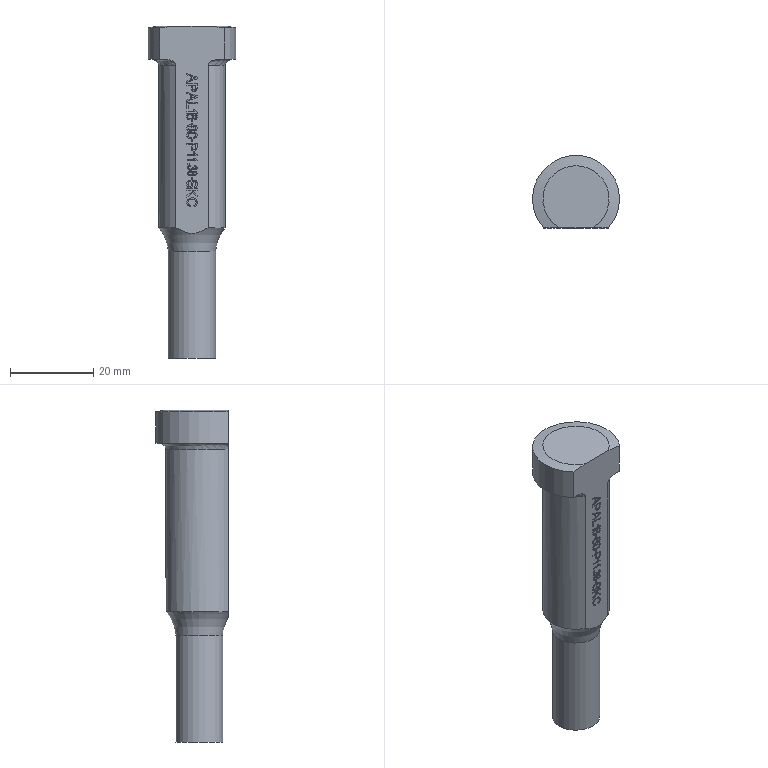Part | NX | features MI_APAL_0252 2 | 1 solid | 235 faces | box 21 x 17.5 x 80 mm | volume 13784 mm3 | plane 159 | cylinder 47 | spline 27 | cone 1 | torus 1 | commonest cylinder face diameters 0.787 x2 0.868 x2 0.984 x2 1.172 x2 1.454 x2 0.678 x1